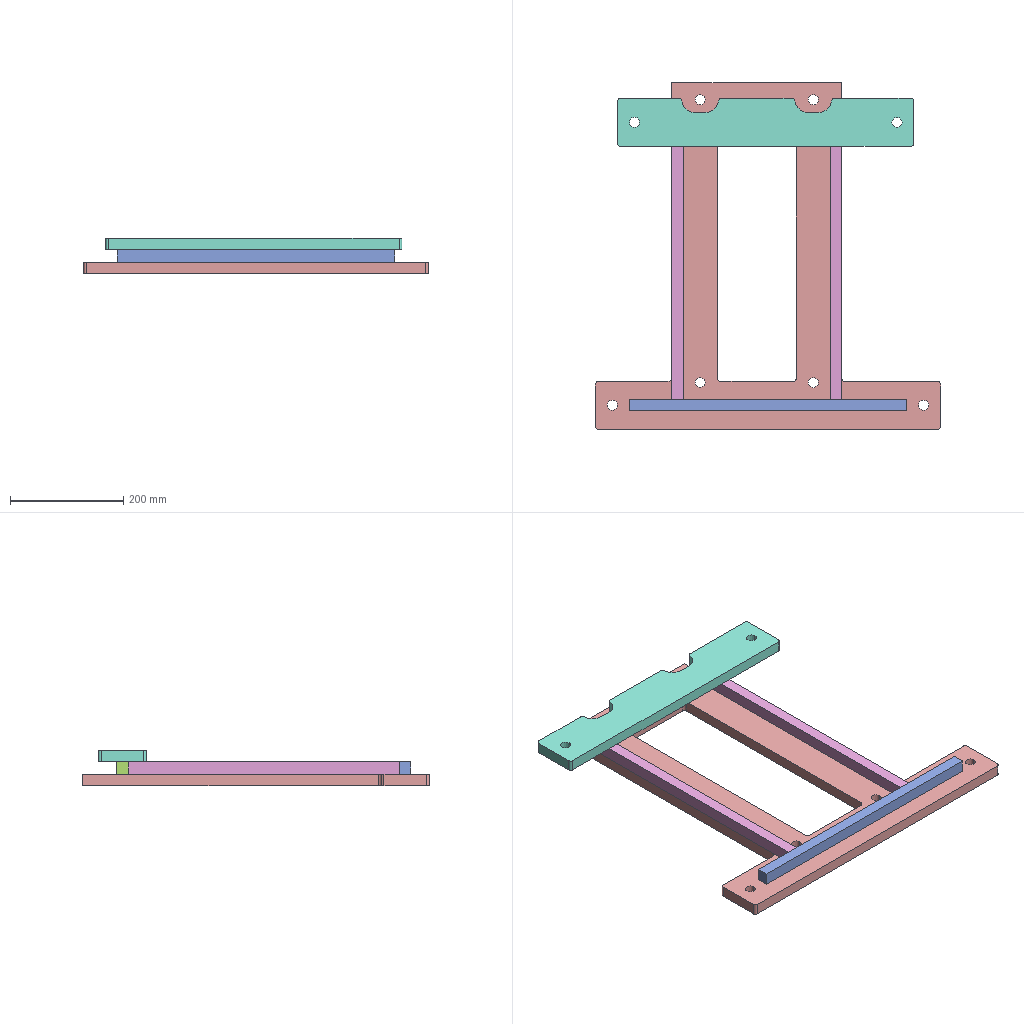Assembly | SolidWorks | 5 different items | 6 placed | box 610 x 612 x 62 mm
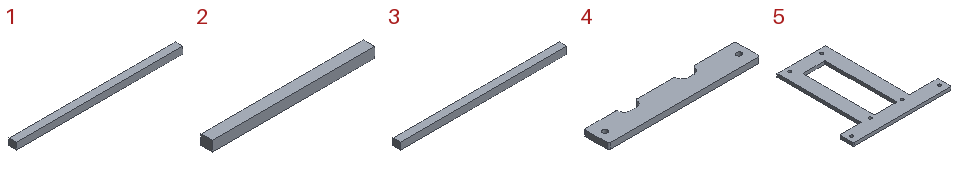Parts list (item | quantity | size | volume | features):
1 | x1 | 490 x 22 x 20 mm | 215600 mm3 | features Extrusion 1
2 | x1 | 318 x 22 x 20 mm | 139920 mm3 | features Extrusion 1
3 | x2 | 480 x 22 x 20 mm | 211200 mm3 | features Extrusion 1
4 | x1 | 524 x 85 x 20 mm | 823491 mm3 | features Extrusion 1
5 | x1 | 610 x 612.5 x 20 mm | 2918678 mm3 | features Extrusion 1
Mates (type | each side: item.copy, entity, surface, feature):
Coincident | 5.1 face plane Boss-Extrude1 | assembly face
DistanceDim | assembly face | 5.1 face plane Boss-Extrude1
Coincident | 5.1 face plane Boss-Extrude1 | 1.1 face plane Boss-Extrude1
Coincident | 5.1 face plane Boss-Extrude1 | 2.1 face plane Boss-Extrude1
Coincident | 5.1 face plane Boss-Extrude1 | 3.1 face plane Boss-Extrude1 | 2 times
Coincident | 5.1 face plane Boss-Extrude1 | 3.2 face plane Boss-Extrude1 | 2 times
Coincident | 1.1 face plane Boss-Extrude1 | 3.2 face plane Boss-Extrude1
Coincident | 1.1 face plane Boss-Extrude1 | 3.1 face plane Boss-Extrude1
DistanceDim | 1.1 face plane Boss-Extrude1 | 5.1 face plane Boss-Extrude1 | 2 times
Coincident | 2.1 face plane Boss-Extrude1 | 3.1 face plane Boss-Extrude1
Coincident | 2.1 face plane Boss-Extrude1 | 3.2 face plane Boss-Extrude1
Coincident | 3.2 face plane Boss-Extrude1 | 4.1 face plane Boss-Extrude1
Parallel | 5.1 face plane Boss-Extrude1 | 4.1 face plane Boss-Extrude1
DistanceDim | 5.1 face plane Boss-Extrude1 | 4.1 face plane Boss-Extrude1
DistanceDim | 4.1 face plane Boss-Extrude1 | 5.1 face plane Boss-Extrude1